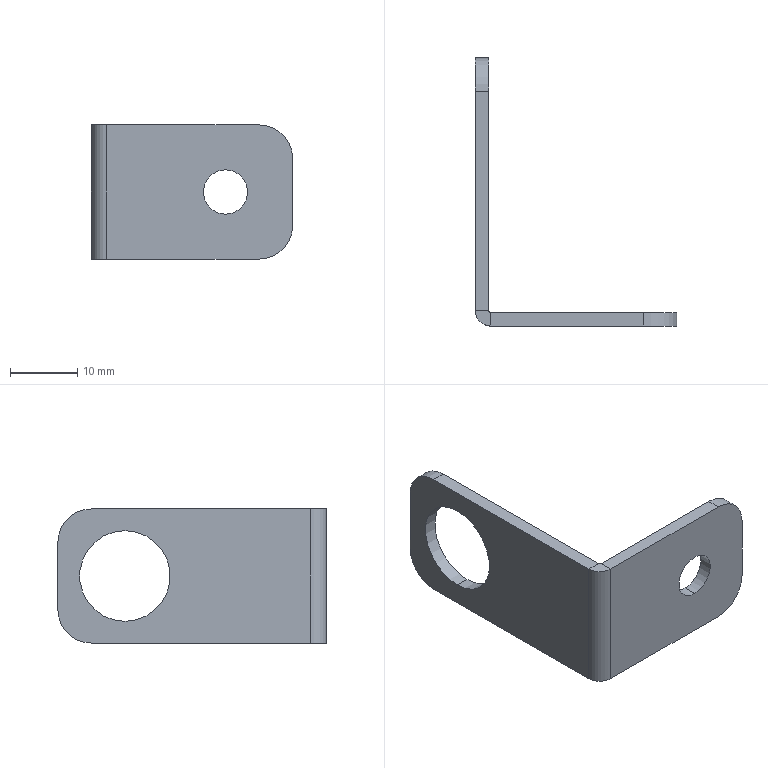Part | SolidWorks | features Fillet 1, FlatPattern 1, HoleWzd 1, ICE 1, SMBaseFlange 1, SheetMetal 1 | 1 solid | 22 faces | box 30 x 40 x 20 mm | volume 2300 mm3 | plane 12 | cylinder 10 | commonest cylinder face diameters 10 x4 6.6 x2 13.5 x2 0.6 x1 4.6 x1
STEP:
#1=CARTESIAN_POINT('',(20.,0.,13.3));
#2=VERTEX_POINT('',#1);
#3=CARTESIAN_POINT('',(20.,0.,6.7));
#4=VERTEX_POINT('',#3);
#5=CARTESIAN_POINT('',(20.,0.,10.));
#6=DIRECTION('',(0.,-1.,0.));
#7=DIRECTION('',(0.,0.,-1.));
#8=AXIS2_PLACEMENT_3D('',#5,#6,#7);
#9=CIRCLE('',#8,3.3);
#10=EDGE_CURVE('',#2,#4,#9,.T.);
#11=ORIENTED_EDGE('',*,*,#10,.T.);
#12=CARTESIAN_POINT('',(20.,2.,6.7));
#13=VERTEX_POINT('',#12);
#14=CARTESIAN_POINT('',(20.,2.,6.7));
#15=DIRECTION('',(0.,1.,0.));
#16=VECTOR('',#15,1000.);
#17=LINE('',#14,#16);
#18=EDGE_CURVE('',#4,#13,#17,.T.);
#19=ORIENTED_EDGE('',*,*,#18,.T.);
#20=CARTESIAN_POINT('',(20.,2.,13.3));
#21=VERTEX_POINT('',#20);
#22=CARTESIAN_POINT('',(20.,2.,10.));
#23=DIRECTION('',(0.,1.,0.));
#24=DIRECTION('',(0.,0.,1.));
#25=AXIS2_PLACEMENT_3D('',#22,#23,#24);
#26=CIRCLE('',#25,3.3);
#27=EDGE_CURVE('',#13,#21,#26,.T.);
#28=ORIENTED_EDGE('',*,*,#27,.T.);
#29=CARTESIAN_POINT('',(20.,2.,13.3));
#30=DIRECTION('',(0.,1.,0.));
#31=VECTOR('',#30,1000.);
#32=LINE('',#29,#31);
#33=EDGE_CURVE('',#2,#21,#32,.T.);
#34=ORIENTED_EDGE('',*,*,#33,.F.);
#35=EDGE_LOOP('',(#11,#19,#28,#34));
#36=FACE_OUTER_BOUND('',#35,.T.);
#37=CARTESIAN_POINT('',(20.,2.,10.));
#38=DIRECTION('',(0.,1.,0.));
#39=DIRECTION('',(0.,0.,1.));
#40=AXIS2_PLACEMENT_3D('',#37,#38,#39);
#41=CYLINDRICAL_SURFACE('',#40,3.3);
#42=ADVANCED_FACE('',(#36),#41,.F.);
#43=CARTESIAN_POINT('',(0.,30.,3.25));
#44=VERTEX_POINT('',#43);
#45=CARTESIAN_POINT('',(0.,30.,16.75));
#46=VERTEX_POINT('',#45);
#47=CARTESIAN_POINT('',(0.,30.,10.));
#48=DIRECTION('',(-1.,0.,0.));
#49=DIRECTION('',(0.,0.,1.));
#50=AXIS2_PLACEMENT_3D('',#47,#48,#49);
#51=CIRCLE('',#50,6.75);
#52=EDGE_CURVE('',#44,#46,#51,.T.);
#53=ORIENTED_EDGE('',*,*,#52,.T.);
#54=CARTESIAN_POINT('',(2.,30.,16.75));
#55=VERTEX_POINT('',#54);
#56=CARTESIAN_POINT('',(-8.,30.,16.75));
#57=DIRECTION('',(1.,0.,0.));
#58=VECTOR('',#57,1000.);
#59=LINE('',#56,#58);
#60=EDGE_CURVE('',#46,#55,#59,.T.);
#61=ORIENTED_EDGE('',*,*,#60,.T.);
#62=CARTESIAN_POINT('',(2.,30.,3.25));
#63=VERTEX_POINT('',#62);
#64=CARTESIAN_POINT('',(2.,30.,10.));
#65=DIRECTION('',(1.,0.,0.));
#66=DIRECTION('',(0.,0.,-1.));
#67=AXIS2_PLACEMENT_3D('',#64,#65,#66);
#68=CIRCLE('',#67,6.75);
#69=EDGE_CURVE('',#55,#63,#68,.T.);
#70=ORIENTED_EDGE('',*,*,#69,.T.);
#71=CARTESIAN_POINT('',(-8.,30.,3.25));
#72=DIRECTION('',(1.,0.,0.));
#73=VECTOR('',#72,1000.);
#74=LINE('',#71,#73);
#75=EDGE_CURVE('',#44,#63,#74,.T.);
#76=ORIENTED_EDGE('',*,*,#75,.F.);
#77=EDGE_LOOP('',(#53,#61,#70,#76));
#78=FACE_OUTER_BOUND('',#77,.T.);
#79=CARTESIAN_POINT('',(-8.,30.,10.));
#80=DIRECTION('',(1.,0.,0.));
#81=DIRECTION('',(0.,0.,-1.));
#82=AXIS2_PLACEMENT_3D('',#79,#80,#81);
#83=CYLINDRICAL_SURFACE('',#82,6.75);
#84=ADVANCED_FACE('',(#78),#83,.F.);
#85=CARTESIAN_POINT('',(0.,2.3,20.));
#86=VERTEX_POINT('',#85);
#87=CARTESIAN_POINT('',(2.,2.3,20.));
#88=VERTEX_POINT('',#87);
#89=CARTESIAN_POINT('',(0.,2.3,20.));
#90=DIRECTION('',(1.,0.,0.));
#91=VECTOR('',#90,1000.);
#92=LINE('',#89,#91);
#93=EDGE_CURVE('',#86,#88,#92,.T.);
#94=ORIENTED_EDGE('',*,*,#93,.F.);
#95=CARTESIAN_POINT('',(2.3,0.,20.));
#96=VERTEX_POINT('',#95);
#97=CARTESIAN_POINT('',(2.3,2.3,20.));
#98=DIRECTION('',(0.,0.,-1.));
#99=DIRECTION('',(1.,0.,0.));
#100=AXIS2_PLACEMENT_3D('',#97,#98,#99);
#101=CIRCLE('',#100,2.3);
#102=EDGE_CURVE('',#96,#86,#101,.T.);
#103=ORIENTED_EDGE('',*,*,#102,.F.);
#104=CARTESIAN_POINT('',(2.3,2.,20.));
#105=VERTEX_POINT('',#104);
#106=CARTESIAN_POINT('',(2.3,2.,20.));
#107=DIRECTION('',(0.,-1.,0.));
#108=VECTOR('',#107,1000.);
#109=LINE('',#106,#108);
#110=EDGE_CURVE('',#105,#96,#109,.T.);
#111=ORIENTED_EDGE('',*,*,#110,.F.);
#112=CARTESIAN_POINT('',(2.3,2.3,20.));
#113=DIRECTION('',(0.,0.,-1.));
#114=DIRECTION('',(1.,0.,0.));
#115=AXIS2_PLACEMENT_3D('',#112,#113,#114);
#116=CIRCLE('',#115,0.3);
#117=EDGE_CURVE('',#105,#88,#116,.T.);
#118=ORIENTED_EDGE('',*,*,#117,.T.);
#119=EDGE_LOOP('',(#94,#103,#111,#118));
#120=FACE_OUTER_BOUND('',#119,.T.);
#121=CARTESIAN_POINT('',(0.,2.3,20.));
#122=DIRECTION('',(0.,0.,1.));
#123=DIRECTION('',(1.,0.,0.));
#124=AXIS2_PLACEMENT_3D('',#121,#122,#123);
#125=PLANE('',#124);
#126=ADVANCED_FACE('',(#120),#125,.T.);
#127=CARTESIAN_POINT('',(2.,35.,20.));
#128=VERTEX_POINT('',#127);
#129=CARTESIAN_POINT('',(2.,0.,20.));
#130=DIRECTION('',(0.,1.,0.));
#131=VECTOR('',#130,1000.);
#132=LINE('',#129,#131);
#133=EDGE_CURVE('',#88,#128,#132,.T.);
#134=ORIENTED_EDGE('',*,*,#133,.T.);
#135=CARTESIAN_POINT('',(0.,35.,20.));
#136=VERTEX_POINT('',#135);
#137=CARTESIAN_POINT('',(2.3,35.,20.));
#138=DIRECTION('',(-1.,0.,0.));
#139=VECTOR('',#138,1000.);
#140=LINE('',#137,#139);
#141=EDGE_CURVE('',#128,#136,#140,.T.);
#142=ORIENTED_EDGE('',*,*,#141,.T.);
#143=CARTESIAN_POINT('',(0.,0.,20.));
#144=DIRECTION('',(0.,1.,0.));
#145=VECTOR('',#144,1000.);
#146=LINE('',#143,#145);
#147=EDGE_CURVE('',#86,#136,#146,.T.);
#148=ORIENTED_EDGE('',*,*,#147,.F.);
#149=ORIENTED_EDGE('',*,*,#93,.T.);
#150=EDGE_LOOP('',(#134,#142,#148,#149));
#151=FACE_OUTER_BOUND('',#150,.T.);
#152=CARTESIAN_POINT('',(2.3,2.,20.));
#153=DIRECTION('',(0.,0.,1.));
#154=DIRECTION('',(1.,0.,0.));
#155=AXIS2_PLACEMENT_3D('',#152,#153,#154);
#156=PLANE('',#155);
#157=ADVANCED_FACE('',(#151),#156,.T.);
#158=CARTESIAN_POINT('',(2.3,0.,0.));
#159=VERTEX_POINT('',#158);
#160=CARTESIAN_POINT('',(2.3,2.,0.));
#161=VERTEX_POINT('',#160);
#162=CARTESIAN_POINT('',(2.3,0.,0.));
#163=DIRECTION('',(0.,1.,0.));
#164=VECTOR('',#163,1000.);
#165=LINE('',#162,#164);
#166=EDGE_CURVE('',#159,#161,#165,.T.);
#167=ORIENTED_EDGE('',*,*,#166,.F.);
#168=CARTESIAN_POINT('',(0.,2.3,0.));
#169=VERTEX_POINT('',#168);
#170=CARTESIAN_POINT('',(2.3,2.3,0.));
#171=DIRECTION('',(0.,0.,-1.));
#172=DIRECTION('',(1.,0.,0.));
#173=AXIS2_PLACEMENT_3D('',#170,#171,#172);
#174=CIRCLE('',#173,2.3);
#175=EDGE_CURVE('',#159,#169,#174,.T.);
#176=ORIENTED_EDGE('',*,*,#175,.T.);
#177=CARTESIAN_POINT('',(2.,2.3,0.));
#178=VERTEX_POINT('',#177);
#179=CARTESIAN_POINT('',(2.,2.3,0.));
#180=DIRECTION('',(-1.,0.,0.));
#181=VECTOR('',#180,1000.);
#182=LINE('',#179,#181);
#183=EDGE_CURVE('',#178,#169,#182,.T.);
#184=ORIENTED_EDGE('',*,*,#183,.F.);
#185=CARTESIAN_POINT('',(2.3,2.3,0.));
#186=DIRECTION('',(0.,0.,-1.));
#187=DIRECTION('',(1.,0.,0.));
#188=AXIS2_PLACEMENT_3D('',#185,#186,#187);
#189=CIRCLE('',#188,0.3);
#190=EDGE_CURVE('',#161,#178,#189,.T.);
#191=ORIENTED_EDGE('',*,*,#190,.F.);
#192=EDGE_LOOP('',(#167,#176,#184,#191));
#193=FACE_OUTER_BOUND('',#192,.T.);
#194=CARTESIAN_POINT('',(2.3,0.,0.));
#195=DIRECTION('',(0.,0.,-1.));
#196=DIRECTION('',(-1.,0.,0.));
#197=AXIS2_PLACEMENT_3D('',#194,#195,#196);
#198=PLANE('',#197);
#199=ADVANCED_FACE('',(#193),#198,.T.);
#200=CARTESIAN_POINT('',(25.,2.,0.));
#201=VERTEX_POINT('',#200);
#202=CARTESIAN_POINT('',(30.,2.,0.));
#203=DIRECTION('',(-1.,0.,0.));
#204=VECTOR('',#203,1000.);
#205=LINE('',#202,#204);
#206=EDGE_CURVE('',#201,#161,#205,.T.);
#207=ORIENTED_EDGE('',*,*,#206,.F.);
#208=CARTESIAN_POINT('',(25.,0.,0.));
#209=VERTEX_POINT('',#208);
#210=CARTESIAN_POINT('',(25.,2.3,0.));
#211=DIRECTION('',(0.,-1.,0.));
#212=VECTOR('',#211,1000.);
#213=LINE('',#210,#212);
#214=EDGE_CURVE('',#201,#209,#213,.T.);
#215=ORIENTED_EDGE('',*,*,#214,.T.);
#216=CARTESIAN_POINT('',(30.,0.,0.));
#217=DIRECTION('',(-1.,0.,0.));
#218=VECTOR('',#217,1000.);
#219=LINE('',#216,#218);
#220=EDGE_CURVE('',#209,#159,#219,.T.);
#221=ORIENTED_EDGE('',*,*,#220,.T.);
#222=ORIENTED_EDGE('',*,*,#166,.T.);
#223=EDGE_LOOP('',(#207,#215,#221,#222));
#224=FACE_OUTER_BOUND('',#223,.T.);
#225=CARTESIAN_POINT('',(2.,2.3,0.));
#226=DIRECTION('',(0.,0.,-1.));
#227=DIRECTION('',(-1.,0.,0.));
#228=AXIS2_PLACEMENT_3D('',#225,#226,#227);
#229=PLANE('',#228);
#230=ADVANCED_FACE('',(#224),#229,.T.);
#231=CARTESIAN_POINT('',(2.,30.,10.));
#232=DIRECTION('',(1.,0.,0.));
#233=DIRECTION('',(0.,0.,-1.));
#234=AXIS2_PLACEMENT_3D('',#231,#232,#233);
#235=CIRCLE('',#234,6.75);
#236=EDGE_CURVE('',#63,#55,#235,.T.);
#237=ORIENTED_EDGE('',*,*,#236,.F.);
#238=ORIENTED_EDGE('',*,*,#69,.F.);
#239=EDGE_LOOP('',(#237,#238));
#240=FACE_BOUND('',#239,.T.);
#241=CARTESIAN_POINT('',(2.,35.,0.));
#242=VERTEX_POINT('',#241);
#243=CARTESIAN_POINT('',(2.,0.,0.));
#244=DIRECTION('',(0.,1.,0.));
#245=VECTOR('',#244,1000.);
#246=LINE('',#243,#245);
#247=EDGE_CURVE('',#178,#242,#246,.T.);
#248=ORIENTED_EDGE('',*,*,#247,.T.);
#249=CARTESIAN_POINT('',(2.,40.,5.));
#250=VERTEX_POINT('',#249);
#251=CARTESIAN_POINT('',(2.,35.,5.));
#252=DIRECTION('',(1.,0.,0.));
#253=DIRECTION('',(0.,0.,1.));
#254=AXIS2_PLACEMENT_3D('',#251,#252,#253);
#255=CIRCLE('',#254,5.);
#256=EDGE_CURVE('',#242,#250,#255,.T.);
#257=ORIENTED_EDGE('',*,*,#256,.T.);
#258=CARTESIAN_POINT('',(2.,40.,15.));
#259=VERTEX_POINT('',#258);
#260=CARTESIAN_POINT('',(2.,40.,20.));
#261=DIRECTION('',(0.,0.,-1.));
#262=VECTOR('',#261,1000.);
#263=LINE('',#260,#262);
#264=EDGE_CURVE('',#259,#250,#263,.T.);
#265=ORIENTED_EDGE('',*,*,#264,.F.);
#266=CARTESIAN_POINT('',(2.,35.,15.));
#267=DIRECTION('',(1.,0.,0.));
#268=DIRECTION('',(0.,0.,1.));
#269=AXIS2_PLACEMENT_3D('',#266,#267,#268);
#270=CIRCLE('',#269,5.);
#271=EDGE_CURVE('',#259,#128,#270,.T.);
#272=ORIENTED_EDGE('',*,*,#271,.T.);
#273=ORIENTED_EDGE('',*,*,#133,.F.);
#274=CARTESIAN_POINT('',(2.,2.3,20.));
#275=DIRECTION('',(0.,0.,-1.));
#276=VECTOR('',#275,1000.);
#277=LINE('',#274,#276);
#278=EDGE_CURVE('',#88,#178,#277,.T.);
#279=ORIENTED_EDGE('',*,*,#278,.T.);
#280=EDGE_LOOP('',(#248,#257,#265,#272,#273,#279));
#281=FACE_OUTER_BOUND('',#280,.T.);
#282=CARTESIAN_POINT('',(2.,0.,20.));
#283=DIRECTION('',(-1.,0.,0.));
#284=DIRECTION('',(0.,0.,1.));
#285=AXIS2_PLACEMENT_3D('',#282,#283,#284);
#286=PLANE('',#285);
#287=ADVANCED_FACE('',(#240,#281),#286,.F.);
#288=ORIENTED_EDGE('',*,*,#264,.T.);
#289=CARTESIAN_POINT('',(0.,40.,5.));
#290=VERTEX_POINT('',#289);
#291=CARTESIAN_POINT('',(0.,40.,5.));
#292=DIRECTION('',(-1.,0.,0.));
#293=VECTOR('',#292,1000.);
#294=LINE('',#291,#293);
#295=EDGE_CURVE('',#250,#290,#294,.T.);
#296=ORIENTED_EDGE('',*,*,#295,.T.);
#297=CARTESIAN_POINT('',(0.,40.,15.));
#298=VERTEX_POINT('',#297);
#299=CARTESIAN_POINT('',(0.,40.,20.));
#300=DIRECTION('',(0.,0.,-1.));
#301=VECTOR('',#300,1000.);
#302=LINE('',#299,#301);
#303=EDGE_CURVE('',#298,#290,#302,.T.);
#304=ORIENTED_EDGE('',*,*,#303,.F.);
#305=CARTESIAN_POINT('',(0.,40.,15.));
#306=DIRECTION('',(1.,0.,0.));
#307=VECTOR('',#306,1000.);
#308=LINE('',#305,#307);
#309=EDGE_CURVE('',#298,#259,#308,.T.);
#310=ORIENTED_EDGE('',*,*,#309,.T.);
#311=EDGE_LOOP('',(#288,#296,#304,#310));
#312=FACE_OUTER_BOUND('',#311,.T.);
#313=CARTESIAN_POINT('',(0.,40.,20.));
#314=DIRECTION('',(0.,1.,0.));
#315=DIRECTION('',(0.,0.,1.));
#316=AXIS2_PLACEMENT_3D('',#313,#314,#315);
#317=PLANE('',#316);
#318=ADVANCED_FACE('',(#312),#317,.T.);
#319=ORIENTED_EDGE('',*,*,#52,.F.);
#320=CARTESIAN_POINT('',(0.,30.,10.));
#321=DIRECTION('',(-1.,0.,0.));
#322=DIRECTION('',(0.,0.,1.));
#323=AXIS2_PLACEMENT_3D('',#320,#321,#322);
#324=CIRCLE('',#323,6.75);
#325=EDGE_CURVE('',#46,#44,#324,.T.);
#326=ORIENTED_EDGE('',*,*,#325,.F.);
#327=EDGE_LOOP('',(#319,#326));
#328=FACE_BOUND('',#327,.T.);
#329=ORIENTED_EDGE('',*,*,#303,.T.);
#330=CARTESIAN_POINT('',(0.,35.,0.));
#331=VERTEX_POINT('',#330);
#332=CARTESIAN_POINT('',(0.,35.,5.));
#333=DIRECTION('',(-1.,0.,0.));
#334=DIRECTION('',(0.,0.,1.));
#335=AXIS2_PLACEMENT_3D('',#332,#333,#334);
#336=CIRCLE('',#335,5.);
#337=EDGE_CURVE('',#290,#331,#336,.T.);
#338=ORIENTED_EDGE('',*,*,#337,.T.);
#339=CARTESIAN_POINT('',(0.,0.,0.));
#340=DIRECTION('',(0.,1.,0.));
#341=VECTOR('',#340,1000.);
#342=LINE('',#339,#341);
#343=EDGE_CURVE('',#169,#331,#342,.T.);
#344=ORIENTED_EDGE('',*,*,#343,.F.);
#345=CARTESIAN_POINT('',(0.,2.3,20.));
#346=DIRECTION('',(0.,0.,-1.));
#347=VECTOR('',#346,1000.);
#348=LINE('',#345,#347);
#349=EDGE_CURVE('',#86,#169,#348,.T.);
#350=ORIENTED_EDGE('',*,*,#349,.F.);
#351=ORIENTED_EDGE('',*,*,#147,.T.);
#352=CARTESIAN_POINT('',(0.,35.,15.));
#353=DIRECTION('',(-1.,0.,0.));
#354=DIRECTION('',(0.,0.,1.));
#355=AXIS2_PLACEMENT_3D('',#352,#353,#354);
#356=CIRCLE('',#355,5.);
#357=EDGE_CURVE('',#136,#298,#356,.T.);
#358=ORIENTED_EDGE('',*,*,#357,.T.);
#359=EDGE_LOOP('',(#329,#338,#344,#350,#351,#358));
#360=FACE_OUTER_BOUND('',#359,.T.);
#361=CARTESIAN_POINT('',(0.,0.,20.));
#362=DIRECTION('',(-1.,0.,0.));
#363=DIRECTION('',(0.,0.,1.));
#364=AXIS2_PLACEMENT_3D('',#361,#362,#363);
#365=PLANE('',#364);
#366=ADVANCED_FACE('',(#328,#360),#365,.T.);
#367=ORIENTED_EDGE('',*,*,#175,.F.);
#368=CARTESIAN_POINT('',(2.3,0.,20.));
#369=DIRECTION('',(0.,0.,-1.));
#370=VECTOR('',#369,1000.);
#371=LINE('',#368,#370);
#372=EDGE_CURVE('',#96,#159,#371,.T.);
#373=ORIENTED_EDGE('',*,*,#372,.F.);
#374=ORIENTED_EDGE('',*,*,#102,.T.);
#375=ORIENTED_EDGE('',*,*,#349,.T.);
#376=EDGE_LOOP('',(#367,#373,#374,#375));
#377=FACE_OUTER_BOUND('',#376,.T.);
#378=CARTESIAN_POINT('',(2.3,2.3,20.));
#379=DIRECTION('',(0.,0.,-1.));
#380=DIRECTION('',(-1.,0.,0.));
#381=AXIS2_PLACEMENT_3D('',#378,#379,#380);
#382=CYLINDRICAL_SURFACE('',#381,2.3);
#383=ADVANCED_FACE('',(#377),#382,.T.);
#384=ORIENTED_EDGE('',*,*,#10,.F.);
#385=CARTESIAN_POINT('',(20.,0.,10.));
#386=DIRECTION('',(0.,-1.,0.));
#387=DIRECTION('',(0.,0.,-1.));
#388=AXIS2_PLACEMENT_3D('',#385,#386,#387);
#389=CIRCLE('',#388,3.3);
#390=EDGE_CURVE('',#4,#2,#389,.T.);
#391=ORIENTED_EDGE('',*,*,#390,.F.);
#392=EDGE_LOOP('',(#384,#391));
#393=FACE_BOUND('',#392,.T.);
#394=CARTESIAN_POINT('',(30.,0.,15.));
#395=VERTEX_POINT('',#394);
#396=CARTESIAN_POINT('',(30.,0.,5.));
#397=VERTEX_POINT('',#396);
#398=CARTESIAN_POINT('',(30.,0.,20.));
#399=DIRECTION('',(0.,0.,-1.));
#400=VECTOR('',#399,1000.);
#401=LINE('',#398,#400);
#402=EDGE_CURVE('',#395,#397,#401,.T.);
#403=ORIENTED_EDGE('',*,*,#402,.F.);
#404=CARTESIAN_POINT('',(25.,0.,20.));
#405=VERTEX_POINT('',#404);
#406=CARTESIAN_POINT('',(25.,0.,15.));
#407=DIRECTION('',(0.,-1.,0.));
#408=DIRECTION('',(0.,0.,-1.));
#409=AXIS2_PLACEMENT_3D('',#406,#407,#408);
#410=CIRCLE('',#409,5.);
#411=EDGE_CURVE('',#395,#405,#410,.T.);
#412=ORIENTED_EDGE('',*,*,#411,.T.);
#413=CARTESIAN_POINT('',(30.,0.,20.));
#414=DIRECTION('',(-1.,0.,0.));
#415=VECTOR('',#414,1000.);
#416=LINE('',#413,#415);
#417=EDGE_CURVE('',#405,#96,#416,.T.);
#418=ORIENTED_EDGE('',*,*,#417,.T.);
#419=ORIENTED_EDGE('',*,*,#372,.T.);
#420=ORIENTED_EDGE('',*,*,#220,.F.);
#421=CARTESIAN_POINT('',(25.,0.,5.));
#422=DIRECTION('',(0.,-1.,0.));
#423=DIRECTION('',(0.,0.,-1.));
#424=AXIS2_PLACEMENT_3D('',#421,#422,#423);
#425=CIRCLE('',#424,5.);
#426=EDGE_CURVE('',#209,#397,#425,.T.);
#427=ORIENTED_EDGE('',*,*,#426,.T.);
#428=EDGE_LOOP('',(#403,#412,#418,#419,#420,#427));
#429=FACE_OUTER_BOUND('',#428,.T.);
#430=CARTESIAN_POINT('',(30.,0.,20.));
#431=DIRECTION('',(0.,-1.,0.));
#432=DIRECTION('',(0.,0.,-1.));
#433=AXIS2_PLACEMENT_3D('',#430,#431,#432);
#434=PLANE('',#433);
#435=ADVANCED_FACE('',(#393,#429),#434,.T.);
#436=CARTESIAN_POINT('',(30.,2.,15.));
#437=VERTEX_POINT('',#436);
#438=CARTESIAN_POINT('',(30.,2.,5.));
#439=VERTEX_POINT('',#438);
#440=CARTESIAN_POINT('',(30.,2.,20.));
#441=DIRECTION('',(0.,0.,-1.));
#442=VECTOR('',#441,1000.);
#443=LINE('',#440,#442);
#444=EDGE_CURVE('',#437,#439,#443,.T.);
#445=ORIENTED_EDGE('',*,*,#444,.F.);
#446=CARTESIAN_POINT('',(30.,2.,15.));
#447=DIRECTION('',(0.,-1.,0.));
#448=VECTOR('',#447,1000.);
#449=LINE('',#446,#448);
#450=EDGE_CURVE('',#437,#395,#449,.T.);
#451=ORIENTED_EDGE('',*,*,#450,.T.);
#452=ORIENTED_EDGE('',*,*,#402,.T.);
#453=CARTESIAN_POINT('',(30.,2.,5.));
#454=DIRECTION('',(0.,1.,0.));
#455=VECTOR('',#454,1000.);
#456=LINE('',#453,#455);
#457=EDGE_CURVE('',#397,#439,#456,.T.);
#458=ORIENTED_EDGE('',*,*,#457,.T.);
#459=EDGE_LOOP('',(#445,#451,#452,#458));
#460=FACE_OUTER_BOUND('',#459,.T.);
#461=CARTESIAN_POINT('',(30.,2.,20.));
#462=DIRECTION('',(1.,0.,0.));
#463=DIRECTION('',(0.,0.,-1.));
#464=AXIS2_PLACEMENT_3D('',#461,#462,#463);
#465=PLANE('',#464);
#466=ADVANCED_FACE('',(#460),#465,.T.);
#467=CARTESIAN_POINT('',(20.,2.,10.));
#468=DIRECTION('',(0.,1.,0.));
#469=DIRECTION('',(0.,0.,1.));
#470=AXIS2_PLACEMENT_3D('',#467,#468,#469);
#471=CIRCLE('',#470,3.3);
#472=EDGE_CURVE('',#21,#13,#471,.T.);
#473=ORIENTED_EDGE('',*,*,#472,.F.);
#474=ORIENTED_EDGE('',*,*,#27,.F.);
#475=EDGE_LOOP('',(#473,#474));
#476=FACE_BOUND('',#475,.T.);
#477=CARTESIAN_POINT('',(25.,2.,20.));
#478=VERTEX_POINT('',#477);
#479=CARTESIAN_POINT('',(30.,2.,20.));
#480=DIRECTION('',(-1.,0.,0.));
#481=VECTOR('',#480,1000.);
#482=LINE('',#479,#481);
#483=EDGE_CURVE('',#478,#105,#482,.T.);
#484=ORIENTED_EDGE('',*,*,#483,.F.);
#485=CARTESIAN_POINT('',(25.,2.,15.));
#486=DIRECTION('',(0.,1.,0.));
#487=DIRECTION('',(0.,0.,-1.));
#488=AXIS2_PLACEMENT_3D('',#485,#486,#487);
#489=CIRCLE('',#488,5.);
#490=EDGE_CURVE('',#478,#437,#489,.T.);
#491=ORIENTED_EDGE('',*,*,#490,.T.);
#492=ORIENTED_EDGE('',*,*,#444,.T.);
#493=CARTESIAN_POINT('',(25.,2.,5.));
#494=DIRECTION('',(0.,1.,0.));
#495=DIRECTION('',(0.,0.,-1.));
#496=AXIS2_PLACEMENT_3D('',#493,#494,#495);
#497=CIRCLE('',#496,5.);
#498=EDGE_CURVE('',#439,#201,#497,.T.);
#499=ORIENTED_EDGE('',*,*,#498,.T.);
#500=ORIENTED_EDGE('',*,*,#206,.T.);
#501=CARTESIAN_POINT('',(2.3,2.,20.));
#502=DIRECTION('',(0.,0.,-1.));
#503=VECTOR('',#502,1000.);
#504=LINE('',#501,#503);
#505=EDGE_CURVE('',#105,#161,#504,.T.);
#506=ORIENTED_EDGE('',*,*,#505,.F.);
#507=EDGE_LOOP('',(#484,#491,#492,#499,#500,#506));
#508=FACE_OUTER_BOUND('',#507,.T.);
#509=CARTESIAN_POINT('',(30.,2.,20.));
#510=DIRECTION('',(0.,-1.,0.));
#511=DIRECTION('',(0.,0.,-1.));
#512=AXIS2_PLACEMENT_3D('',#509,#510,#511);
#513=PLANE('',#512);
#514=ADVANCED_FACE('',(#476,#508),#513,.F.);
#515=ORIENTED_EDGE('',*,*,#190,.T.);
#516=ORIENTED_EDGE('',*,*,#278,.F.);
#517=ORIENTED_EDGE('',*,*,#117,.F.);
#518=ORIENTED_EDGE('',*,*,#505,.T.);
#519=EDGE_LOOP('',(#515,#516,#517,#518));
#520=FACE_OUTER_BOUND('',#519,.T.);
#521=CARTESIAN_POINT('',(2.3,2.3,20.));
#522=DIRECTION('',(0.,0.,-1.));
#523=DIRECTION('',(-1.,0.,0.));
#524=AXIS2_PLACEMENT_3D('',#521,#522,#523);
#525=CYLINDRICAL_SURFACE('',#524,0.3);
#526=ADVANCED_FACE('',(#520),#525,.F.);
#527=ORIENTED_EDGE('',*,*,#417,.F.);
#528=CARTESIAN_POINT('',(25.,2.3,20.));
#529=DIRECTION('',(0.,1.,0.));
#530=VECTOR('',#529,1000.);
#531=LINE('',#528,#530);
#532=EDGE_CURVE('',#405,#478,#531,.T.);
#533=ORIENTED_EDGE('',*,*,#532,.T.);
#534=ORIENTED_EDGE('',*,*,#483,.T.);
#535=ORIENTED_EDGE('',*,*,#110,.T.);
#536=EDGE_LOOP('',(#527,#533,#534,#535));
#537=FACE_OUTER_BOUND('',#536,.T.);
#538=CARTESIAN_POINT('',(2.3,2.3,20.));
#539=DIRECTION('',(0.,0.,1.));
#540=DIRECTION('',(1.,0.,0.));
#541=AXIS2_PLACEMENT_3D('',#538,#539,#540);
#542=PLANE('',#541);
#543=ADVANCED_FACE('',(#537),#542,.T.);
#544=ORIENTED_EDGE('',*,*,#343,.T.);
#545=CARTESIAN_POINT('',(2.,35.,0.));
#546=DIRECTION('',(1.,0.,0.));
#547=VECTOR('',#546,1000.);
#548=LINE('',#545,#547);
#549=EDGE_CURVE('',#331,#242,#548,.T.);
#550=ORIENTED_EDGE('',*,*,#549,.T.);
#551=ORIENTED_EDGE('',*,*,#247,.F.);
#552=ORIENTED_EDGE('',*,*,#183,.T.);
#553=EDGE_LOOP('',(#544,#550,#551,#552));
#554=FACE_OUTER_BOUND('',#553,.T.);
#555=CARTESIAN_POINT('',(2.3,2.3,0.));
#556=DIRECTION('',(0.,0.,1.));
#557=DIRECTION('',(1.,0.,0.));
#558=AXIS2_PLACEMENT_3D('',#555,#556,#557);
#559=PLANE('',#558);
#560=ADVANCED_FACE('',(#554),#559,.F.);
#561=ORIENTED_EDGE('',*,*,#490,.F.);
#562=ORIENTED_EDGE('',*,*,#532,.F.);
#563=ORIENTED_EDGE('',*,*,#411,.F.);
#564=ORIENTED_EDGE('',*,*,#450,.F.);
#565=EDGE_LOOP('',(#561,#562,#563,#564));
#566=FACE_OUTER_BOUND('',#565,.T.);
#567=CARTESIAN_POINT('',(25.,2.,15.));
#568=DIRECTION('',(0.,-1.,0.));
#569=DIRECTION('',(0.,0.,-1.));
#570=AXIS2_PLACEMENT_3D('',#567,#568,#569);
#571=CYLINDRICAL_SURFACE('',#570,5.);
#572=ADVANCED_FACE('',(#566),#571,.T.);
#573=ORIENTED_EDGE('',*,*,#498,.F.);
#574=ORIENTED_EDGE('',*,*,#457,.F.);
#575=ORIENTED_EDGE('',*,*,#426,.F.);
#576=ORIENTED_EDGE('',*,*,#214,.F.);
#577=EDGE_LOOP('',(#573,#574,#575,#576));
#578=FACE_OUTER_BOUND('',#577,.T.);
#579=CARTESIAN_POINT('',(25.,2.3,5.));
#580=DIRECTION('',(0.,-1.,0.));
#581=DIRECTION('',(0.,0.,-1.));
#582=AXIS2_PLACEMENT_3D('',#579,#580,#581);
#583=CYLINDRICAL_SURFACE('',#582,5.);
#584=ADVANCED_FACE('',(#578),#583,.T.);
#585=ORIENTED_EDGE('',*,*,#337,.F.);
#586=ORIENTED_EDGE('',*,*,#295,.F.);
#587=ORIENTED_EDGE('',*,*,#256,.F.);
#588=ORIENTED_EDGE('',*,*,#549,.F.);
#589=EDGE_LOOP('',(#585,#586,#587,#588));
#590=FACE_OUTER_BOUND('',#589,.T.);
#591=CARTESIAN_POINT('',(2.3,35.,5.));
#592=DIRECTION('',(-1.,0.,0.));
#593=DIRECTION('',(0.,0.,1.));
#594=AXIS2_PLACEMENT_3D('',#591,#592,#593);
#595=CYLINDRICAL_SURFACE('',#594,5.);
#596=ADVANCED_FACE('',(#590),#595,.T.);
#597=ORIENTED_EDGE('',*,*,#357,.F.);
#598=ORIENTED_EDGE('',*,*,#141,.F.);
#599=ORIENTED_EDGE('',*,*,#271,.F.);
#600=ORIENTED_EDGE('',*,*,#309,.F.);
#601=EDGE_LOOP('',(#597,#598,#599,#600));
#602=FACE_OUTER_BOUND('',#601,.T.);
#603=CARTESIAN_POINT('',(0.,35.,15.));
#604=DIRECTION('',(1.,0.,0.));
#605=DIRECTION('',(0.,0.,-1.));
#606=AXIS2_PLACEMENT_3D('',#603,#604,#605);
#607=CYLINDRICAL_SURFACE('',#606,5.);
#608=ADVANCED_FACE('',(#602),#607,.T.);
#609=ORIENTED_EDGE('',*,*,#60,.F.);
#610=ORIENTED_EDGE('',*,*,#325,.T.);
#611=ORIENTED_EDGE('',*,*,#75,.T.);
#612=ORIENTED_EDGE('',*,*,#236,.T.);
#613=EDGE_LOOP('',(#609,#610,#611,#612));
#614=FACE_OUTER_BOUND('',#613,.T.);
#615=CARTESIAN_POINT('',(-8.,30.,10.));
#616=DIRECTION('',(1.,0.,0.));
#617=DIRECTION('',(0.,0.,-1.));
#618=AXIS2_PLACEMENT_3D('',#615,#616,#617);
#619=CYLINDRICAL_SURFACE('',#618,6.75);
#620=ADVANCED_FACE('',(#614),#619,.F.);
#621=ORIENTED_EDGE('',*,*,#18,.F.);
#622=ORIENTED_EDGE('',*,*,#390,.T.);
#623=ORIENTED_EDGE('',*,*,#33,.T.);
#624=ORIENTED_EDGE('',*,*,#472,.T.);
#625=EDGE_LOOP('',(#621,#622,#623,#624));
#626=FACE_OUTER_BOUND('',#625,.T.);
#627=CARTESIAN_POINT('',(20.,2.,10.));
#628=DIRECTION('',(0.,1.,0.));
#629=DIRECTION('',(0.,0.,1.));
#630=AXIS2_PLACEMENT_3D('',#627,#628,#629);
#631=CYLINDRICAL_SURFACE('',#630,3.3);
#632=ADVANCED_FACE('',(#626),#631,.F.);
#633=CLOSED_SHELL('',(#42,#84,#126,#157,#199,#230,#287,#318,#366,#383,#435,#466,#514,#526,#543,#560,#572,#584,#596,#608,#620,#632));
#634=MANIFOLD_SOLID_BREP('',#633);
#635=CARTESIAN_POINT('',(0.,0.,0.));
#636=DIRECTION('',(0.,0.,1.));
#637=DIRECTION('',(1.,0.,0.));
#638=AXIS2_PLACEMENT_3D('',#635,#636,#637);
#639=(LENGTH_UNIT()NAMED_UNIT(*)SI_UNIT(.MILLI.,.METRE.));
#640=UNCERTAINTY_MEASURE_WITH_UNIT(LENGTH_MEASURE(0.00001),#639,'','');
#641=(NAMED_UNIT(*)PLANE_ANGLE_UNIT()SI_UNIT($,.RADIAN.));
#642=(NAMED_UNIT(*)SI_UNIT($,.STERADIAN.)SOLID_ANGLE_UNIT());
#643=(GEOMETRIC_REPRESENTATION_CONTEXT(3)GLOBAL_UNCERTAINTY_ASSIGNED_CONTEXT((#640))GLOBAL_UNIT_ASSIGNED_CONTEXT((#639,#641,#642))REPRESENTATION_CONTEXT('',''));
#644=ADVANCED_BREP_SHAPE_REPRESENTATION('',(#634,#638),#643);